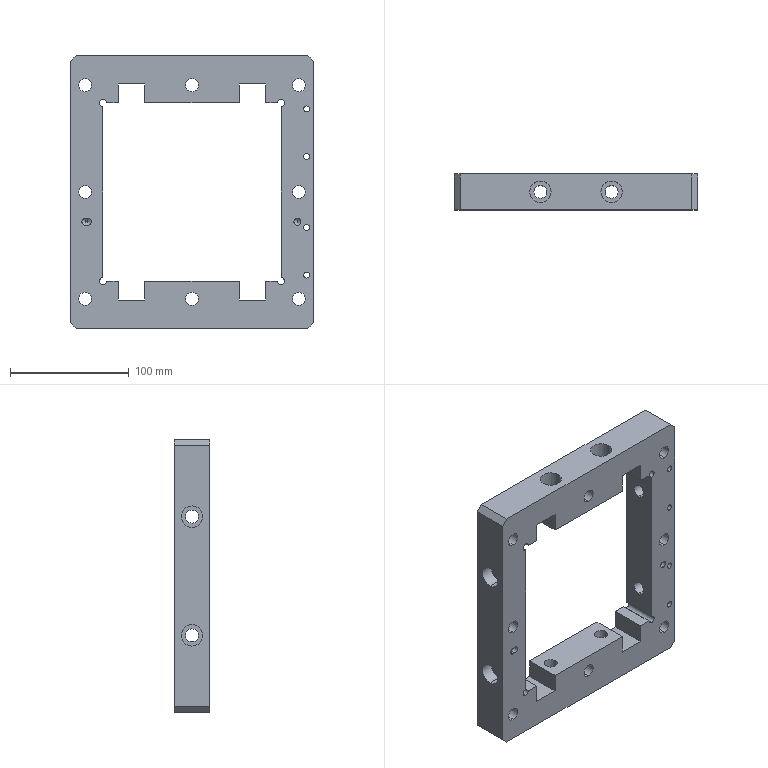Part | SolidWorks | features HoleWzd 9, Chamfer 1, Cut 1, Extrusion 1 | 1 solid | 136 faces | box 205 x 30 x 230 mm | volume 608627 mm3 | cylinder 82 | plane 50 | cone 4 | commonest cylinder face diameters 11 x32 18 x32 6 x10 5 x8